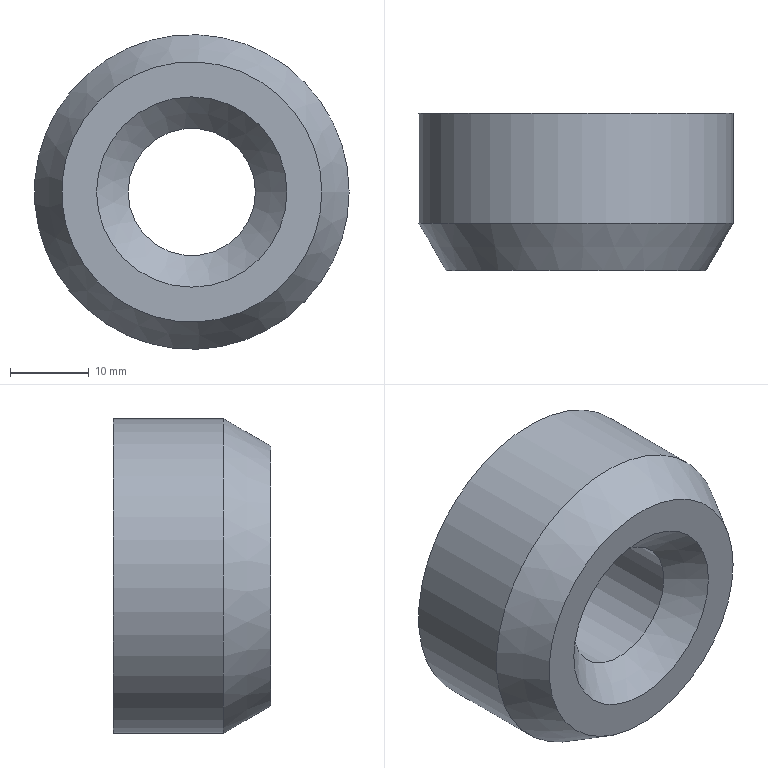Part | NX | features solid 2 | 1 solid | 7 faces | box 40 x 20 x 40 mm | volume 19289 mm3 | cone 3 | plane 2 | cylinder 2 | commonest cylinder face diameters 16.2 x1 40 x1
STEP:
#1=CARTESIAN_POINT('',(801.536,330.,145.));
#2=VERTEX_POINT('',#1);
#3=CARTESIAN_POINT('',(785.,330.,145.));
#4=DIRECTION('',(0.,1.,0.));
#5=DIRECTION('',(1.,0.,0.));
#6=AXIS2_PLACEMENT_3D('',#3,#4,#5);
#7=CIRCLE('',#6,16.536);
#8=EDGE_CURVE('',#2,#2,#7,.T.);
#9=ORIENTED_EDGE('',*,*,#8,.F.);
#10=EDGE_LOOP('',(#9));
#11=FACE_BOUND('',#10,.T.);
#12=CARTESIAN_POINT('',(797.1,330.,145.));
#13=VERTEX_POINT('',#12);
#14=CARTESIAN_POINT('',(785.,330.,145.));
#15=DIRECTION('',(0.,1.,0.));
#16=DIRECTION('',(1.,0.,0.));
#17=AXIS2_PLACEMENT_3D('',#14,#15,#16);
#18=CIRCLE('',#17,12.1);
#19=EDGE_CURVE('',#13,#13,#18,.F.);
#20=ORIENTED_EDGE('',*,*,#19,.F.);
#21=EDGE_LOOP('',(#20));
#22=FACE_BOUND('',#21,.T.);
#23=CARTESIAN_POINT('',(785.,330.,145.));
#24=DIRECTION('',(0.,-1.,0.));
#25=DIRECTION('',(1.,0.,0.));
#26=AXIS2_PLACEMENT_3D('',#23,#24,#25);
#27=PLANE('',#26);
#28=ADVANCED_FACE('',(#11,#22),#27,.T.);
#29=CARTESIAN_POINT('',(776.1,350.,145.));
#30=VERTEX_POINT('',#29);
#31=CARTESIAN_POINT('',(785.,350.,145.));
#32=DIRECTION('',(0.,-1.,0.));
#33=DIRECTION('',(-1.,0.,0.));
#34=AXIS2_PLACEMENT_3D('',#31,#32,#33);
#35=CIRCLE('',#34,8.9);
#36=EDGE_CURVE('',#30,#30,#35,.F.);
#37=ORIENTED_EDGE('',*,*,#36,.F.);
#38=EDGE_LOOP('',(#37));
#39=FACE_BOUND('',#38,.T.);
#40=CARTESIAN_POINT('',(805.,350.,145.));
#41=VERTEX_POINT('',#40);
#42=CARTESIAN_POINT('',(785.,350.,145.));
#43=DIRECTION('',(0.,1.,0.));
#44=DIRECTION('',(1.,0.,0.));
#45=AXIS2_PLACEMENT_3D('',#42,#43,#44);
#46=CIRCLE('',#45,20.);
#47=EDGE_CURVE('',#41,#41,#46,.T.);
#48=ORIENTED_EDGE('',*,*,#47,.T.);
#49=EDGE_LOOP('',(#48));
#50=FACE_BOUND('',#49,.T.);
#51=CARTESIAN_POINT('',(785.,350.,145.));
#52=DIRECTION('',(0.,1.,0.));
#53=DIRECTION('',(-1.,0.,0.));
#54=AXIS2_PLACEMENT_3D('',#51,#52,#53);
#55=PLANE('',#54);
#56=ADVANCED_FACE('',(#39,#50),#55,.T.);
#57=CARTESIAN_POINT('',(805.,336.,145.));
#58=VERTEX_POINT('',#57);
#59=CARTESIAN_POINT('',(785.,336.,145.));
#60=DIRECTION('',(0.,1.,0.));
#61=DIRECTION('',(1.,0.,0.));
#62=AXIS2_PLACEMENT_3D('',#59,#60,#61);
#63=CIRCLE('',#62,20.);
#64=EDGE_CURVE('',#58,#58,#63,.F.);
#65=ORIENTED_EDGE('',*,*,#64,.F.);
#66=EDGE_LOOP('',(#65));
#67=FACE_BOUND('',#66,.T.);
#68=ORIENTED_EDGE('',*,*,#47,.F.);
#69=EDGE_LOOP('',(#68));
#70=FACE_BOUND('',#69,.T.);
#71=CARTESIAN_POINT('',(785.,350.,145.));
#72=DIRECTION('',(0.,-1.,0.));
#73=DIRECTION('',(1.,0.,0.));
#74=AXIS2_PLACEMENT_3D('',#71,#72,#73);
#75=CYLINDRICAL_SURFACE('',#74,20.);
#76=ADVANCED_FACE('',(#67,#70),#75,.T.);
#77=CARTESIAN_POINT('',(793.1,334.,145.));
#78=VERTEX_POINT('',#77);
#79=CARTESIAN_POINT('',(785.,334.,145.));
#80=DIRECTION('',(0.,1.,0.));
#81=DIRECTION('',(1.,0.,0.));
#82=AXIS2_PLACEMENT_3D('',#79,#80,#81);
#83=CIRCLE('',#82,8.1);
#84=EDGE_CURVE('',#78,#78,#83,.T.);
#85=ORIENTED_EDGE('',*,*,#84,.F.);
#86=EDGE_LOOP('',(#85));
#87=FACE_BOUND('',#86,.T.);
#88=CARTESIAN_POINT('',(776.9,349.2,145.));
#89=VERTEX_POINT('',#88);
#90=CARTESIAN_POINT('',(785.,349.2,145.));
#91=DIRECTION('',(0.,-1.,0.));
#92=DIRECTION('',(-1.,0.,0.));
#93=AXIS2_PLACEMENT_3D('',#90,#91,#92);
#94=CIRCLE('',#93,8.1);
#95=EDGE_CURVE('',#89,#89,#94,.T.);
#96=ORIENTED_EDGE('',*,*,#95,.F.);
#97=EDGE_LOOP('',(#96));
#98=FACE_BOUND('',#97,.T.);
#99=CARTESIAN_POINT('',(785.,350.,145.));
#100=DIRECTION('',(0.,-1.,0.));
#101=DIRECTION('',(1.,0.,0.));
#102=AXIS2_PLACEMENT_3D('',#99,#100,#101);
#103=CYLINDRICAL_SURFACE('',#102,8.1);
#104=ADVANCED_FACE('',(#87,#98),#103,.F.);
#105=ORIENTED_EDGE('',*,*,#95,.T.);
#106=EDGE_LOOP('',(#105));
#107=FACE_BOUND('',#106,.T.);
#108=ORIENTED_EDGE('',*,*,#36,.T.);
#109=EDGE_LOOP('',(#108));
#110=FACE_BOUND('',#109,.T.);
#111=CARTESIAN_POINT('',(785.,350.,145.));
#112=DIRECTION('',(0.,1.,0.));
#113=DIRECTION('',(-1.,0.,0.));
#114=AXIS2_PLACEMENT_3D('',#111,#112,#113);
#115=CONICAL_SURFACE('',#114,8.9,0.7854);
#116=ADVANCED_FACE('',(#107,#110),#115,.F.);
#117=ORIENTED_EDGE('',*,*,#84,.T.);
#118=EDGE_LOOP('',(#117));
#119=FACE_BOUND('',#118,.T.);
#120=ORIENTED_EDGE('',*,*,#19,.T.);
#121=EDGE_LOOP('',(#120));
#122=FACE_BOUND('',#121,.T.);
#123=CARTESIAN_POINT('',(785.,330.,145.));
#124=DIRECTION('',(0.,-1.,0.));
#125=DIRECTION('',(1.,0.,0.));
#126=AXIS2_PLACEMENT_3D('',#123,#124,#125);
#127=CONICAL_SURFACE('',#126,12.1,0.7854);
#128=ADVANCED_FACE('',(#119,#122),#127,.F.);
#129=ORIENTED_EDGE('',*,*,#8,.T.);
#130=EDGE_LOOP('',(#129));
#131=FACE_BOUND('',#130,.T.);
#132=ORIENTED_EDGE('',*,*,#64,.T.);
#133=EDGE_LOOP('',(#132));
#134=FACE_BOUND('',#133,.T.);
#135=CARTESIAN_POINT('',(785.,336.,145.));
#136=DIRECTION('',(0.,1.,0.));
#137=DIRECTION('',(-1.,0.,0.));
#138=AXIS2_PLACEMENT_3D('',#135,#136,#137);
#139=CONICAL_SURFACE('',#138,20.,0.5236);
#140=ADVANCED_FACE('',(#131,#134),#139,.T.);
#141=CLOSED_SHELL('',(#28,#56,#76,#104,#116,#128,#140));
#142=MANIFOLD_SOLID_BREP('',#141);
#143=(LENGTH_UNIT()NAMED_UNIT(*)SI_UNIT(.MILLI.,.METRE.));
#144=UNCERTAINTY_MEASURE_WITH_UNIT(LENGTH_MEASURE(0.00001),#143,'','');
#145=(NAMED_UNIT(*)PLANE_ANGLE_UNIT()SI_UNIT($,.RADIAN.));
#146=(NAMED_UNIT(*)SI_UNIT($,.STERADIAN.)SOLID_ANGLE_UNIT());
#147=(GEOMETRIC_REPRESENTATION_CONTEXT(3)GLOBAL_UNCERTAINTY_ASSIGNED_CONTEXT((#144))GLOBAL_UNIT_ASSIGNED_CONTEXT((#143,#145,#146))REPRESENTATION_CONTEXT('',''));
#148=ADVANCED_BREP_SHAPE_REPRESENTATION('',(#142),#147);